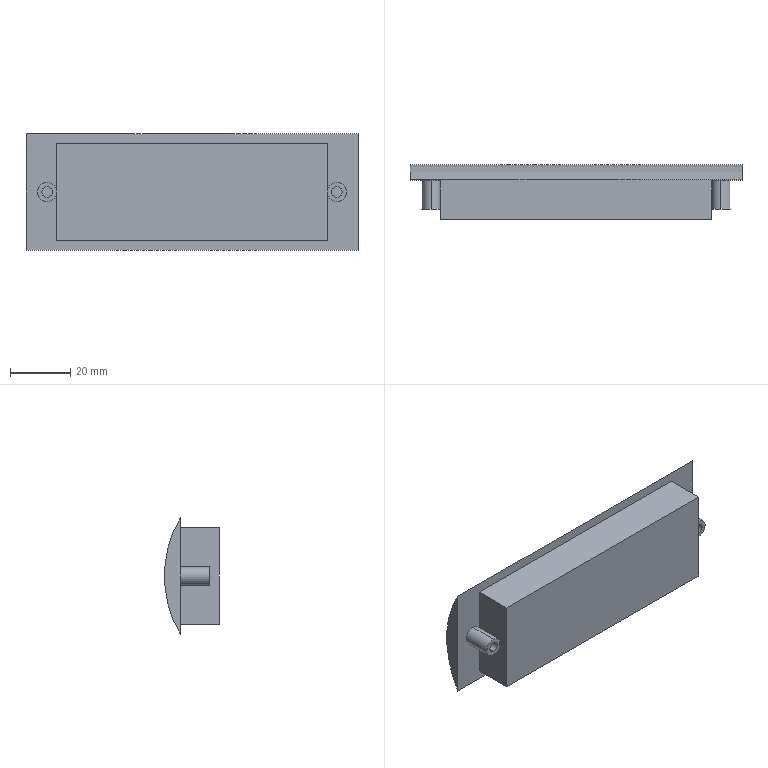Part | STEP file | LE-LLS-96A_LE0314002343 | 1 solid | 23 faces | box 110 x 18.2 x 38.5 mm | volume 52750 mm3 | plane 12 | cylinder 11 | commonest cylinder face diameters 6.3 x6 3.5 x4 76.462 x1
STEP:
#1=CARTESIAN_POINT('',(48.,-9.75,3.15));
#2=VERTEX_POINT('',#1);
#3=CARTESIAN_POINT('',(48.,-9.75,-3.15));
#4=VERTEX_POINT('',#3);
#5=CARTESIAN_POINT('',(48.,-9.75,0.));
#6=DIRECTION('',(0.,1.,0.));
#7=DIRECTION('',(0.,0.,1.));
#8=AXIS2_PLACEMENT_3D('',#5,#6,#7);
#9=CIRCLE('',#8,3.15);
#10=EDGE_CURVE('',#2,#4,#9,.T.);
#11=ORIENTED_EDGE('',*,*,#10,.T.);
#12=CARTESIAN_POINT('',(48.,0.,-3.15));
#13=VERTEX_POINT('',#12);
#14=CARTESIAN_POINT('',(48.,-9.75,-3.15));
#15=DIRECTION('',(0.,1.,0.));
#16=VECTOR('',#15,1000.);
#17=LINE('',#14,#16);
#18=EDGE_CURVE('',#4,#13,#17,.T.);
#19=ORIENTED_EDGE('',*,*,#18,.T.);
#20=CARTESIAN_POINT('',(48.,0.,3.15));
#21=VERTEX_POINT('',#20);
#22=CARTESIAN_POINT('',(48.,0.,0.));
#23=DIRECTION('',(0.,1.,0.));
#24=DIRECTION('',(0.,0.,1.));
#25=AXIS2_PLACEMENT_3D('',#22,#23,#24);
#26=CIRCLE('',#25,3.15);
#27=EDGE_CURVE('',#21,#13,#26,.T.);
#28=ORIENTED_EDGE('',*,*,#27,.F.);
#29=CARTESIAN_POINT('',(48.,-9.75,3.15));
#30=DIRECTION('',(0.,1.,0.));
#31=VECTOR('',#30,1000.);
#32=LINE('',#29,#31);
#33=EDGE_CURVE('',#2,#21,#32,.T.);
#34=ORIENTED_EDGE('',*,*,#33,.F.);
#35=EDGE_LOOP('',(#11,#19,#28,#34));
#36=FACE_OUTER_BOUND('',#35,.T.);
#37=CARTESIAN_POINT('',(48.,-9.75,0.));
#38=DIRECTION('',(0.,1.,0.));
#39=DIRECTION('',(0.,0.,1.));
#40=AXIS2_PLACEMENT_3D('',#37,#38,#39);
#41=CYLINDRICAL_SURFACE('',#40,3.15);
#42=ADVANCED_FACE('',(#36),#41,.T.);
#43=CARTESIAN_POINT('',(45.,-9.75,0.9605));
#44=VERTEX_POINT('',#43);
#45=CARTESIAN_POINT('',(48.,-9.75,0.));
#46=DIRECTION('',(0.,1.,0.));
#47=DIRECTION('',(0.,0.,1.));
#48=AXIS2_PLACEMENT_3D('',#45,#46,#47);
#49=CIRCLE('',#48,3.15);
#50=EDGE_CURVE('',#44,#2,#49,.T.);
#51=ORIENTED_EDGE('',*,*,#50,.T.);
#52=ORIENTED_EDGE('',*,*,#33,.T.);
#53=CARTESIAN_POINT('',(45.,0.,0.9605));
#54=VERTEX_POINT('',#53);
#55=CARTESIAN_POINT('',(48.,0.,0.));
#56=DIRECTION('',(0.,1.,0.));
#57=DIRECTION('',(0.,0.,1.));
#58=AXIS2_PLACEMENT_3D('',#55,#56,#57);
#59=CIRCLE('',#58,3.15);
#60=EDGE_CURVE('',#54,#21,#59,.T.);
#61=ORIENTED_EDGE('',*,*,#60,.F.);
#62=CARTESIAN_POINT('',(45.,-13.,0.9605));
#63=DIRECTION('',(0.,-1.,0.));
#64=VECTOR('',#63,1000.);
#65=LINE('',#62,#64);
#66=EDGE_CURVE('',#54,#44,#65,.T.);
#67=ORIENTED_EDGE('',*,*,#66,.T.);
#68=EDGE_LOOP('',(#51,#52,#61,#67));
#69=FACE_OUTER_BOUND('',#68,.T.);
#70=CARTESIAN_POINT('',(48.,-9.75,0.));
#71=DIRECTION('',(0.,1.,0.));
#72=DIRECTION('',(0.,0.,1.));
#73=AXIS2_PLACEMENT_3D('',#70,#71,#72);
#74=CYLINDRICAL_SURFACE('',#73,3.15);
#75=ADVANCED_FACE('',(#69),#74,.T.);
#76=CARTESIAN_POINT('',(-45.,-9.75,-0.9605));
#77=VERTEX_POINT('',#76);
#78=CARTESIAN_POINT('',(-48.,-9.75,-3.15));
#79=VERTEX_POINT('',#78);
#80=CARTESIAN_POINT('',(-48.,-9.75,0.));
#81=DIRECTION('',(0.,1.,0.));
#82=DIRECTION('',(0.,0.,1.));
#83=AXIS2_PLACEMENT_3D('',#80,#81,#82);
#84=CIRCLE('',#83,3.15);
#85=EDGE_CURVE('',#77,#79,#84,.T.);
#86=ORIENTED_EDGE('',*,*,#85,.T.);
#87=CARTESIAN_POINT('',(-48.,0.,-3.15));
#88=VERTEX_POINT('',#87);
#89=CARTESIAN_POINT('',(-48.,-9.75,-3.15));
#90=DIRECTION('',(0.,1.,0.));
#91=VECTOR('',#90,1000.);
#92=LINE('',#89,#91);
#93=EDGE_CURVE('',#79,#88,#92,.T.);
#94=ORIENTED_EDGE('',*,*,#93,.T.);
#95=CARTESIAN_POINT('',(-45.,0.,-0.9605));
#96=VERTEX_POINT('',#95);
#97=CARTESIAN_POINT('',(-48.,0.,0.));
#98=DIRECTION('',(0.,1.,0.));
#99=DIRECTION('',(0.,0.,1.));
#100=AXIS2_PLACEMENT_3D('',#97,#98,#99);
#101=CIRCLE('',#100,3.15);
#102=EDGE_CURVE('',#96,#88,#101,.T.);
#103=ORIENTED_EDGE('',*,*,#102,.F.);
#104=CARTESIAN_POINT('',(-45.,-13.,-0.9605));
#105=DIRECTION('',(0.,-1.,0.));
#106=VECTOR('',#105,1000.);
#107=LINE('',#104,#106);
#108=EDGE_CURVE('',#96,#77,#107,.T.);
#109=ORIENTED_EDGE('',*,*,#108,.T.);
#110=EDGE_LOOP('',(#86,#94,#103,#109));
#111=FACE_OUTER_BOUND('',#110,.T.);
#112=CARTESIAN_POINT('',(-48.,-9.75,0.));
#113=DIRECTION('',(0.,1.,0.));
#114=DIRECTION('',(0.,0.,1.));
#115=AXIS2_PLACEMENT_3D('',#112,#113,#114);
#116=CYLINDRICAL_SURFACE('',#115,3.15);
#117=ADVANCED_FACE('',(#111),#116,.T.);
#118=ORIENTED_EDGE('',*,*,#93,.F.);
#119=CARTESIAN_POINT('',(-48.,-9.75,3.15));
#120=VERTEX_POINT('',#119);
#121=CARTESIAN_POINT('',(-48.,-9.75,0.));
#122=DIRECTION('',(0.,1.,0.));
#123=DIRECTION('',(0.,0.,1.));
#124=AXIS2_PLACEMENT_3D('',#121,#122,#123);
#125=CIRCLE('',#124,3.15);
#126=EDGE_CURVE('',#79,#120,#125,.T.);
#127=ORIENTED_EDGE('',*,*,#126,.T.);
#128=CARTESIAN_POINT('',(-48.,0.,3.15));
#129=VERTEX_POINT('',#128);
#130=CARTESIAN_POINT('',(-48.,-9.75,3.15));
#131=DIRECTION('',(0.,1.,0.));
#132=VECTOR('',#131,1000.);
#133=LINE('',#130,#132);
#134=EDGE_CURVE('',#120,#129,#133,.T.);
#135=ORIENTED_EDGE('',*,*,#134,.T.);
#136=CARTESIAN_POINT('',(-48.,0.,0.));
#137=DIRECTION('',(0.,1.,0.));
#138=DIRECTION('',(0.,0.,1.));
#139=AXIS2_PLACEMENT_3D('',#136,#137,#138);
#140=CIRCLE('',#139,3.15);
#141=EDGE_CURVE('',#88,#129,#140,.T.);
#142=ORIENTED_EDGE('',*,*,#141,.F.);
#143=EDGE_LOOP('',(#118,#127,#135,#142));
#144=FACE_OUTER_BOUND('',#143,.T.);
#145=CARTESIAN_POINT('',(-48.,-9.75,0.));
#146=DIRECTION('',(0.,1.,0.));
#147=DIRECTION('',(0.,0.,1.));
#148=AXIS2_PLACEMENT_3D('',#145,#146,#147);
#149=CYLINDRICAL_SURFACE('',#148,3.15);
#150=ADVANCED_FACE('',(#144),#149,.T.);
#151=CARTESIAN_POINT('',(48.,0.,1.75));
#152=VERTEX_POINT('',#151);
#153=CARTESIAN_POINT('',(48.,0.,-1.75));
#154=VERTEX_POINT('',#153);
#155=CARTESIAN_POINT('',(48.,0.,0.));
#156=DIRECTION('',(0.,-1.,0.));
#157=DIRECTION('',(0.,0.,-1.));
#158=AXIS2_PLACEMENT_3D('',#155,#156,#157);
#159=CIRCLE('',#158,1.75);
#160=EDGE_CURVE('',#152,#154,#159,.T.);
#161=ORIENTED_EDGE('',*,*,#160,.F.);
#162=CARTESIAN_POINT('',(48.,-9.75,1.75));
#163=VERTEX_POINT('',#162);
#164=CARTESIAN_POINT('',(48.,0.,1.75));
#165=DIRECTION('',(0.,-1.,0.));
#166=VECTOR('',#165,1000.);
#167=LINE('',#164,#166);
#168=EDGE_CURVE('',#152,#163,#167,.T.);
#169=ORIENTED_EDGE('',*,*,#168,.T.);
#170=CARTESIAN_POINT('',(48.,-9.75,-1.75));
#171=VERTEX_POINT('',#170);
#172=CARTESIAN_POINT('',(48.,-9.75,0.));
#173=DIRECTION('',(0.,1.,0.));
#174=DIRECTION('',(0.,0.,-1.));
#175=AXIS2_PLACEMENT_3D('',#172,#173,#174);
#176=CIRCLE('',#175,1.75);
#177=EDGE_CURVE('',#171,#163,#176,.T.);
#178=ORIENTED_EDGE('',*,*,#177,.F.);
#179=CARTESIAN_POINT('',(48.,0.,-1.75));
#180=DIRECTION('',(0.,-1.,0.));
#181=VECTOR('',#180,1000.);
#182=LINE('',#179,#181);
#183=EDGE_CURVE('',#154,#171,#182,.T.);
#184=ORIENTED_EDGE('',*,*,#183,.F.);
#185=EDGE_LOOP('',(#161,#169,#178,#184));
#186=FACE_OUTER_BOUND('',#185,.T.);
#187=CARTESIAN_POINT('',(48.,0.,0.));
#188=DIRECTION('',(0.,-1.,0.));
#189=DIRECTION('',(0.,0.,-1.));
#190=AXIS2_PLACEMENT_3D('',#187,#188,#189);
#191=CYLINDRICAL_SURFACE('',#190,1.75);
#192=ADVANCED_FACE('',(#186),#191,.F.);
#193=CARTESIAN_POINT('',(-48.,0.,1.75));
#194=VERTEX_POINT('',#193);
#195=CARTESIAN_POINT('',(-48.,0.,-1.75));
#196=VERTEX_POINT('',#195);
#197=CARTESIAN_POINT('',(-48.,0.,0.));
#198=DIRECTION('',(0.,-1.,0.));
#199=DIRECTION('',(0.,0.,-1.));
#200=AXIS2_PLACEMENT_3D('',#197,#198,#199);
#201=CIRCLE('',#200,1.75);
#202=EDGE_CURVE('',#194,#196,#201,.T.);
#203=ORIENTED_EDGE('',*,*,#202,.F.);
#204=CARTESIAN_POINT('',(-48.,-9.75,1.75));
#205=VERTEX_POINT('',#204);
#206=CARTESIAN_POINT('',(-48.,0.,1.75));
#207=DIRECTION('',(0.,-1.,0.));
#208=VECTOR('',#207,1000.);
#209=LINE('',#206,#208);
#210=EDGE_CURVE('',#194,#205,#209,.T.);
#211=ORIENTED_EDGE('',*,*,#210,.T.);
#212=CARTESIAN_POINT('',(-48.,-9.75,-1.75));
#213=VERTEX_POINT('',#212);
#214=CARTESIAN_POINT('',(-48.,-9.75,0.));
#215=DIRECTION('',(0.,1.,0.));
#216=DIRECTION('',(0.,0.,-1.));
#217=AXIS2_PLACEMENT_3D('',#214,#215,#216);
#218=CIRCLE('',#217,1.75);
#219=EDGE_CURVE('',#213,#205,#218,.T.);
#220=ORIENTED_EDGE('',*,*,#219,.F.);
#221=CARTESIAN_POINT('',(-48.,0.,-1.75));
#222=DIRECTION('',(0.,-1.,0.));
#223=VECTOR('',#222,1000.);
#224=LINE('',#221,#223);
#225=EDGE_CURVE('',#196,#213,#224,.T.);
#226=ORIENTED_EDGE('',*,*,#225,.F.);
#227=EDGE_LOOP('',(#203,#211,#220,#226));
#228=FACE_OUTER_BOUND('',#227,.T.);
#229=CARTESIAN_POINT('',(-48.,0.,0.));
#230=DIRECTION('',(0.,-1.,0.));
#231=DIRECTION('',(0.,0.,-1.));
#232=AXIS2_PLACEMENT_3D('',#229,#230,#231);
#233=CYLINDRICAL_SURFACE('',#232,1.75);
#234=ADVANCED_FACE('',(#228),#233,.F.);
#235=CARTESIAN_POINT('',(55.,0.,-19.25));
#236=VERTEX_POINT('',#235);
#237=CARTESIAN_POINT('',(-55.,0.,-19.25));
#238=VERTEX_POINT('',#237);
#239=CARTESIAN_POINT('',(55.,0.,-19.25));
#240=DIRECTION('',(-1.,0.,0.));
#241=VECTOR('',#240,1000.);
#242=LINE('',#239,#241);
#243=EDGE_CURVE('',#236,#238,#242,.T.);
#244=ORIENTED_EDGE('',*,*,#243,.T.);
#245=CARTESIAN_POINT('',(-55.,0.,19.25));
#246=VERTEX_POINT('',#245);
#247=CARTESIAN_POINT('',(-55.,-33.031,0.));
#248=DIRECTION('',(1.,0.,0.));
#249=DIRECTION('',(0.,-1.,0.));
#250=AXIS2_PLACEMENT_3D('',#247,#248,#249);
#251=CIRCLE('',#250,38.231);
#252=EDGE_CURVE('',#238,#246,#251,.T.);
#253=ORIENTED_EDGE('',*,*,#252,.T.);
#254=CARTESIAN_POINT('',(55.,0.,19.25));
#255=VERTEX_POINT('',#254);
#256=CARTESIAN_POINT('',(55.,0.,19.25));
#257=DIRECTION('',(1.,0.,0.));
#258=VECTOR('',#257,1000.);
#259=LINE('',#256,#258);
#260=EDGE_CURVE('',#246,#255,#259,.T.);
#261=ORIENTED_EDGE('',*,*,#260,.T.);
#262=CARTESIAN_POINT('',(55.,-33.031,0.));
#263=DIRECTION('',(-1.,0.,0.));
#264=DIRECTION('',(0.,-1.,0.));
#265=AXIS2_PLACEMENT_3D('',#262,#263,#264);
#266=CIRCLE('',#265,38.231);
#267=EDGE_CURVE('',#255,#236,#266,.T.);
#268=ORIENTED_EDGE('',*,*,#267,.T.);
#269=EDGE_LOOP('',(#244,#253,#261,#268));
#270=FACE_OUTER_BOUND('',#269,.T.);
#271=CARTESIAN_POINT('',(55.,-33.031,0.));
#272=DIRECTION('',(-1.,0.,0.));
#273=DIRECTION('',(0.,-1.,0.));
#274=AXIS2_PLACEMENT_3D('',#271,#272,#273);
#275=CYLINDRICAL_SURFACE('',#274,38.231);
#276=ADVANCED_FACE('',(#270),#275,.T.);
#277=ORIENTED_EDGE('',*,*,#252,.F.);
#278=CARTESIAN_POINT('',(-55.,0.,0.));
#279=DIRECTION('',(0.,0.,1.));
#280=VECTOR('',#279,1000.);
#281=LINE('',#278,#280);
#282=EDGE_CURVE('',#238,#246,#281,.T.);
#283=ORIENTED_EDGE('',*,*,#282,.T.);
#284=EDGE_LOOP('',(#277,#283));
#285=FACE_OUTER_BOUND('',#284,.T.);
#286=CARTESIAN_POINT('',(-55.,-33.031,0.));
#287=DIRECTION('',(-1.,0.,0.));
#288=DIRECTION('',(0.,0.,1.));
#289=AXIS2_PLACEMENT_3D('',#286,#287,#288);
#290=PLANE('',#289);
#291=ADVANCED_FACE('',(#285),#290,.T.);
#292=ORIENTED_EDGE('',*,*,#60,.T.);
#293=ORIENTED_EDGE('',*,*,#27,.T.);
#294=CARTESIAN_POINT('',(45.,0.,-0.9605));
#295=VERTEX_POINT('',#294);
#296=CARTESIAN_POINT('',(48.,0.,0.));
#297=DIRECTION('',(0.,1.,0.));
#298=DIRECTION('',(0.,0.,1.));
#299=AXIS2_PLACEMENT_3D('',#296,#297,#298);
#300=CIRCLE('',#299,3.15);
#301=EDGE_CURVE('',#13,#295,#300,.T.);
#302=ORIENTED_EDGE('',*,*,#301,.T.);
#303=CARTESIAN_POINT('',(45.,0.,-16.));
#304=VERTEX_POINT('',#303);
#305=CARTESIAN_POINT('',(45.,0.,-19.25));
#306=DIRECTION('',(0.,0.,-1.));
#307=VECTOR('',#306,1000.);
#308=LINE('',#305,#307);
#309=EDGE_CURVE('',#295,#304,#308,.T.);
#310=ORIENTED_EDGE('',*,*,#309,.T.);
#311=CARTESIAN_POINT('',(-45.,0.,-16.));
#312=VERTEX_POINT('',#311);
#313=CARTESIAN_POINT('',(55.,0.,-16.));
#314=DIRECTION('',(-1.,0.,0.));
#315=VECTOR('',#314,1000.);
#316=LINE('',#313,#315);
#317=EDGE_CURVE('',#304,#312,#316,.T.);
#318=ORIENTED_EDGE('',*,*,#317,.T.);
#319=CARTESIAN_POINT('',(-45.,0.,-19.25));
#320=DIRECTION('',(0.,0.,1.));
#321=VECTOR('',#320,1000.);
#322=LINE('',#319,#321);
#323=EDGE_CURVE('',#312,#96,#322,.T.);
#324=ORIENTED_EDGE('',*,*,#323,.T.);
#325=ORIENTED_EDGE('',*,*,#102,.T.);
#326=ORIENTED_EDGE('',*,*,#141,.T.);
#327=CARTESIAN_POINT('',(-45.,0.,0.9605));
#328=VERTEX_POINT('',#327);
#329=CARTESIAN_POINT('',(-48.,0.,0.));
#330=DIRECTION('',(0.,1.,0.));
#331=DIRECTION('',(0.,0.,1.));
#332=AXIS2_PLACEMENT_3D('',#329,#330,#331);
#333=CIRCLE('',#332,3.15);
#334=EDGE_CURVE('',#129,#328,#333,.T.);
#335=ORIENTED_EDGE('',*,*,#334,.T.);
#336=CARTESIAN_POINT('',(-45.,0.,16.));
#337=VERTEX_POINT('',#336);
#338=CARTESIAN_POINT('',(-45.,0.,-19.25));
#339=DIRECTION('',(0.,0.,1.));
#340=VECTOR('',#339,1000.);
#341=LINE('',#338,#340);
#342=EDGE_CURVE('',#328,#337,#341,.T.);
#343=ORIENTED_EDGE('',*,*,#342,.T.);
#344=CARTESIAN_POINT('',(45.,0.,16.));
#345=VERTEX_POINT('',#344);
#346=CARTESIAN_POINT('',(55.,0.,16.));
#347=DIRECTION('',(1.,0.,0.));
#348=VECTOR('',#347,1000.);
#349=LINE('',#346,#348);
#350=EDGE_CURVE('',#337,#345,#349,.T.);
#351=ORIENTED_EDGE('',*,*,#350,.T.);
#352=CARTESIAN_POINT('',(45.,0.,-19.25));
#353=DIRECTION('',(0.,0.,-1.));
#354=VECTOR('',#353,1000.);
#355=LINE('',#352,#354);
#356=EDGE_CURVE('',#345,#54,#355,.T.);
#357=ORIENTED_EDGE('',*,*,#356,.T.);
#358=EDGE_LOOP('',(#292,#293,#302,#310,#318,#324,#325,#326,#335,#343,#351,#357));
#359=FACE_BOUND('',#358,.T.);
#360=ORIENTED_EDGE('',*,*,#260,.F.);
#361=ORIENTED_EDGE('',*,*,#282,.F.);
#362=ORIENTED_EDGE('',*,*,#243,.F.);
#363=CARTESIAN_POINT('',(55.,0.,-19.25));
#364=DIRECTION('',(0.,0.,1.));
#365=VECTOR('',#364,1000.);
#366=LINE('',#363,#365);
#367=EDGE_CURVE('',#236,#255,#366,.T.);
#368=ORIENTED_EDGE('',*,*,#367,.T.);
#369=EDGE_LOOP('',(#360,#361,#362,#368));
#370=FACE_OUTER_BOUND('',#369,.T.);
#371=CARTESIAN_POINT('',(55.,0.,-19.25));
#372=DIRECTION('',(0.,-1.,0.));
#373=DIRECTION('',(1.,0.,0.));
#374=AXIS2_PLACEMENT_3D('',#371,#372,#373);
#375=PLANE('',#374);
#376=ADVANCED_FACE('',(#359,#370),#375,.T.);
#377=ORIENTED_EDGE('',*,*,#267,.F.);
#378=ORIENTED_EDGE('',*,*,#367,.F.);
#379=EDGE_LOOP('',(#377,#378));
#380=FACE_OUTER_BOUND('',#379,.T.);
#381=CARTESIAN_POINT('',(55.,-33.031,0.));
#382=DIRECTION('',(-1.,0.,0.));
#383=DIRECTION('',(0.,0.,1.));
#384=AXIS2_PLACEMENT_3D('',#381,#382,#383);
#385=PLANE('',#384);
#386=ADVANCED_FACE('',(#380),#385,.F.);
#387=CARTESIAN_POINT('',(45.,-13.,16.));
#388=VERTEX_POINT('',#387);
#389=CARTESIAN_POINT('',(45.,-13.,16.));
#390=DIRECTION('',(0.,1.,0.));
#391=VECTOR('',#390,1000.);
#392=LINE('',#389,#391);
#393=EDGE_CURVE('',#388,#345,#392,.T.);
#394=ORIENTED_EDGE('',*,*,#393,.F.);
#395=CARTESIAN_POINT('',(45.,-13.,-16.));
#396=VERTEX_POINT('',#395);
#397=CARTESIAN_POINT('',(45.,-13.,-16.));
#398=DIRECTION('',(0.,0.,1.));
#399=VECTOR('',#398,1000.);
#400=LINE('',#397,#399);
#401=EDGE_CURVE('',#396,#388,#400,.T.);
#402=ORIENTED_EDGE('',*,*,#401,.F.);
#403=CARTESIAN_POINT('',(45.,-13.,-16.));
#404=DIRECTION('',(0.,-1.,0.));
#405=VECTOR('',#404,1000.);
#406=LINE('',#403,#405);
#407=EDGE_CURVE('',#304,#396,#406,.T.);
#408=ORIENTED_EDGE('',*,*,#407,.F.);
#409=ORIENTED_EDGE('',*,*,#309,.F.);
#410=CARTESIAN_POINT('',(45.,-9.75,-0.9605));
#411=VERTEX_POINT('',#410);
#412=CARTESIAN_POINT('',(45.,-13.,-0.9605));
#413=DIRECTION('',(0.,1.,0.));
#414=VECTOR('',#413,1000.);
#415=LINE('',#412,#414);
#416=EDGE_CURVE('',#411,#295,#415,.T.);
#417=ORIENTED_EDGE('',*,*,#416,.F.);
#418=CARTESIAN_POINT('',(45.,-9.75,-16.));
#419=DIRECTION('',(0.,0.,-1.));
#420=VECTOR('',#419,1000.);
#421=LINE('',#418,#420);
#422=EDGE_CURVE('',#44,#411,#421,.T.);
#423=ORIENTED_EDGE('',*,*,#422,.F.);
#424=ORIENTED_EDGE('',*,*,#66,.F.);
#425=ORIENTED_EDGE('',*,*,#356,.F.);
#426=EDGE_LOOP('',(#394,#402,#408,#409,#417,#423,#424,#425));
#427=FACE_OUTER_BOUND('',#426,.T.);
#428=CARTESIAN_POINT('',(45.,-13.,-16.));
#429=DIRECTION('',(-1.,0.,0.));
#430=DIRECTION('',(0.,0.,1.));
#431=AXIS2_PLACEMENT_3D('',#428,#429,#430);
#432=PLANE('',#431);
#433=ADVANCED_FACE('',(#427),#432,.F.);
#434=ORIENTED_EDGE('',*,*,#18,.F.);
#435=CARTESIAN_POINT('',(48.,-9.75,0.));
#436=DIRECTION('',(0.,1.,0.));
#437=DIRECTION('',(0.,0.,1.));
#438=AXIS2_PLACEMENT_3D('',#435,#436,#437);
#439=CIRCLE('',#438,3.15);
#440=EDGE_CURVE('',#4,#411,#439,.T.);
#441=ORIENTED_EDGE('',*,*,#440,.T.);
#442=ORIENTED_EDGE('',*,*,#416,.T.);
#443=ORIENTED_EDGE('',*,*,#301,.F.);
#444=EDGE_LOOP('',(#434,#441,#442,#443));
#445=FACE_OUTER_BOUND('',#444,.T.);
#446=CARTESIAN_POINT('',(48.,-9.75,0.));
#447=DIRECTION('',(0.,1.,0.));
#448=DIRECTION('',(0.,0.,1.));
#449=AXIS2_PLACEMENT_3D('',#446,#447,#448);
#450=CYLINDRICAL_SURFACE('',#449,3.15);
#451=ADVANCED_FACE('',(#445),#450,.T.);
#452=CARTESIAN_POINT('',(-45.,-13.,16.));
#453=VERTEX_POINT('',#452);
#454=CARTESIAN_POINT('',(-45.,-13.,16.));
#455=DIRECTION('',(-1.,0.,0.));
#456=VECTOR('',#455,1000.);
#457=LINE('',#454,#456);
#458=EDGE_CURVE('',#388,#453,#457,.T.);
#459=ORIENTED_EDGE('',*,*,#458,.F.);
#460=ORIENTED_EDGE('',*,*,#393,.T.);
#461=ORIENTED_EDGE('',*,*,#350,.F.);
#462=CARTESIAN_POINT('',(-45.,-13.,16.));
#463=DIRECTION('',(0.,1.,0.));
#464=VECTOR('',#463,1000.);
#465=LINE('',#462,#464);
#466=EDGE_CURVE('',#453,#337,#465,.T.);
#467=ORIENTED_EDGE('',*,*,#466,.F.);
#468=EDGE_LOOP('',(#459,#460,#461,#467));
#469=FACE_OUTER_BOUND('',#468,.T.);
#470=CARTESIAN_POINT('',(-45.,-13.,16.));
#471=DIRECTION('',(0.,0.,-1.));
#472=DIRECTION('',(-1.,0.,0.));
#473=AXIS2_PLACEMENT_3D('',#470,#471,#472);
#474=PLANE('',#473);
#475=ADVANCED_FACE('',(#469),#474,.F.);
#476=ORIENTED_EDGE('',*,*,#323,.F.);
#477=CARTESIAN_POINT('',(-45.,-13.,-16.));
#478=VERTEX_POINT('',#477);
#479=CARTESIAN_POINT('',(-45.,-13.,-16.));
#480=DIRECTION('',(0.,1.,0.));
#481=VECTOR('',#480,1000.);
#482=LINE('',#479,#481);
#483=EDGE_CURVE('',#478,#312,#482,.T.);
#484=ORIENTED_EDGE('',*,*,#483,.F.);
#485=CARTESIAN_POINT('',(-45.,-13.,-16.));
#486=DIRECTION('',(0.,0.,-1.));
#487=VECTOR('',#486,1000.);
#488=LINE('',#485,#487);
#489=EDGE_CURVE('',#453,#478,#488,.T.);
#490=ORIENTED_EDGE('',*,*,#489,.F.);
#491=ORIENTED_EDGE('',*,*,#466,.T.);
#492=ORIENTED_EDGE('',*,*,#342,.F.);
#493=CARTESIAN_POINT('',(-45.,-9.75,0.9605));
#494=VERTEX_POINT('',#493);
#495=CARTESIAN_POINT('',(-45.,-13.,0.9605));
#496=DIRECTION('',(0.,1.,0.));
#497=VECTOR('',#496,1000.);
#498=LINE('',#495,#497);
#499=EDGE_CURVE('',#494,#328,#498,.T.);
#500=ORIENTED_EDGE('',*,*,#499,.F.);
#501=CARTESIAN_POINT('',(-45.,-9.75,-16.));
#502=DIRECTION('',(0.,0.,1.));
#503=VECTOR('',#502,1000.);
#504=LINE('',#501,#503);
#505=EDGE_CURVE('',#77,#494,#504,.T.);
#506=ORIENTED_EDGE('',*,*,#505,.F.);
#507=ORIENTED_EDGE('',*,*,#108,.F.);
#508=EDGE_LOOP('',(#476,#484,#490,#491,#492,#500,#506,#507));
#509=FACE_OUTER_BOUND('',#508,.T.);
#510=CARTESIAN_POINT('',(-45.,-13.,-16.));
#511=DIRECTION('',(1.,0.,0.));
#512=DIRECTION('',(0.,0.,-1.));
#513=AXIS2_PLACEMENT_3D('',#510,#511,#512);
#514=PLANE('',#513);
#515=ADVANCED_FACE('',(#509),#514,.F.);
#516=ORIENTED_EDGE('',*,*,#134,.F.);
#517=CARTESIAN_POINT('',(-48.,-9.75,0.));
#518=DIRECTION('',(0.,1.,0.));
#519=DIRECTION('',(0.,0.,1.));
#520=AXIS2_PLACEMENT_3D('',#517,#518,#519);
#521=CIRCLE('',#520,3.15);
#522=EDGE_CURVE('',#120,#494,#521,.T.);
#523=ORIENTED_EDGE('',*,*,#522,.T.);
#524=ORIENTED_EDGE('',*,*,#499,.T.);
#525=ORIENTED_EDGE('',*,*,#334,.F.);
#526=EDGE_LOOP('',(#516,#523,#524,#525));
#527=FACE_OUTER_BOUND('',#526,.T.);
#528=CARTESIAN_POINT('',(-48.,-9.75,0.));
#529=DIRECTION('',(0.,1.,0.));
#530=DIRECTION('',(0.,0.,1.));
#531=AXIS2_PLACEMENT_3D('',#528,#529,#530);
#532=CYLINDRICAL_SURFACE('',#531,3.15);
#533=ADVANCED_FACE('',(#527),#532,.T.);
#534=CARTESIAN_POINT('',(-45.,-13.,-16.));
#535=DIRECTION('',(1.,0.,0.));
#536=VECTOR('',#535,1000.);
#537=LINE('',#534,#536);
#538=EDGE_CURVE('',#478,#396,#537,.T.);
#539=ORIENTED_EDGE('',*,*,#538,.F.);
#540=ORIENTED_EDGE('',*,*,#483,.T.);
#541=ORIENTED_EDGE('',*,*,#317,.F.);
#542=ORIENTED_EDGE('',*,*,#407,.T.);
#543=EDGE_LOOP('',(#539,#540,#541,#542));
#544=FACE_OUTER_BOUND('',#543,.T.);
#545=CARTESIAN_POINT('',(-45.,-13.,-16.));
#546=DIRECTION('',(0.,0.,1.));
#547=DIRECTION('',(1.,0.,0.));
#548=AXIS2_PLACEMENT_3D('',#545,#546,#547);
#549=PLANE('',#548);
#550=ADVANCED_FACE('',(#544),#549,.F.);
#551=ORIENTED_EDGE('',*,*,#538,.T.);
#552=ORIENTED_EDGE('',*,*,#401,.T.);
#553=ORIENTED_EDGE('',*,*,#458,.T.);
#554=ORIENTED_EDGE('',*,*,#489,.T.);
#555=EDGE_LOOP('',(#551,#552,#553,#554));
#556=FACE_OUTER_BOUND('',#555,.T.);
#557=CARTESIAN_POINT('',(45.,-13.,-16.));
#558=DIRECTION('',(0.,-1.,0.));
#559=DIRECTION('',(0.,0.,-1.));
#560=AXIS2_PLACEMENT_3D('',#557,#558,#559);
#561=PLANE('',#560);
#562=ADVANCED_FACE('',(#556),#561,.T.);
#563=ORIENTED_EDGE('',*,*,#177,.T.);
#564=CARTESIAN_POINT('',(48.,-9.75,0.));
#565=DIRECTION('',(0.,1.,0.));
#566=DIRECTION('',(0.,0.,-1.));
#567=AXIS2_PLACEMENT_3D('',#564,#565,#566);
#568=CIRCLE('',#567,1.75);
#569=EDGE_CURVE('',#163,#171,#568,.T.);
#570=ORIENTED_EDGE('',*,*,#569,.T.);
#571=EDGE_LOOP('',(#563,#570));
#572=FACE_BOUND('',#571,.T.);
#573=ORIENTED_EDGE('',*,*,#50,.F.);
#574=ORIENTED_EDGE('',*,*,#422,.T.);
#575=ORIENTED_EDGE('',*,*,#440,.F.);
#576=ORIENTED_EDGE('',*,*,#10,.F.);
#577=EDGE_LOOP('',(#573,#574,#575,#576));
#578=FACE_OUTER_BOUND('',#577,.T.);
#579=CARTESIAN_POINT('',(48.,-9.75,0.));
#580=DIRECTION('',(0.,-1.,0.));
#581=DIRECTION('',(1.,0.,0.));
#582=AXIS2_PLACEMENT_3D('',#579,#580,#581);
#583=PLANE('',#582);
#584=ADVANCED_FACE('',(#572,#578),#583,.T.);
#585=ORIENTED_EDGE('',*,*,#85,.F.);
#586=ORIENTED_EDGE('',*,*,#505,.T.);
#587=ORIENTED_EDGE('',*,*,#522,.F.);
#588=ORIENTED_EDGE('',*,*,#126,.F.);
#589=EDGE_LOOP('',(#585,#586,#587,#588));
#590=FACE_OUTER_BOUND('',#589,.T.);
#591=ORIENTED_EDGE('',*,*,#219,.T.);
#592=CARTESIAN_POINT('',(-48.,-9.75,0.));
#593=DIRECTION('',(0.,1.,0.));
#594=DIRECTION('',(0.,0.,-1.));
#595=AXIS2_PLACEMENT_3D('',#592,#593,#594);
#596=CIRCLE('',#595,1.75);
#597=EDGE_CURVE('',#205,#213,#596,.T.);
#598=ORIENTED_EDGE('',*,*,#597,.T.);
#599=EDGE_LOOP('',(#591,#598));
#600=FACE_BOUND('',#599,.T.);
#601=CARTESIAN_POINT('',(-48.,-9.75,0.));
#602=DIRECTION('',(0.,-1.,0.));
#603=DIRECTION('',(1.,0.,0.));
#604=AXIS2_PLACEMENT_3D('',#601,#602,#603);
#605=PLANE('',#604);
#606=ADVANCED_FACE('',(#590,#600),#605,.T.);
#607=ORIENTED_EDGE('',*,*,#168,.F.);
#608=CARTESIAN_POINT('',(48.,0.,0.));
#609=DIRECTION('',(0.,-1.,0.));
#610=DIRECTION('',(0.,0.,-1.));
#611=AXIS2_PLACEMENT_3D('',#608,#609,#610);
#612=CIRCLE('',#611,1.75);
#613=EDGE_CURVE('',#154,#152,#612,.T.);
#614=ORIENTED_EDGE('',*,*,#613,.F.);
#615=ORIENTED_EDGE('',*,*,#183,.T.);
#616=ORIENTED_EDGE('',*,*,#569,.F.);
#617=EDGE_LOOP('',(#607,#614,#615,#616));
#618=FACE_OUTER_BOUND('',#617,.T.);
#619=CARTESIAN_POINT('',(48.,0.,0.));
#620=DIRECTION('',(0.,-1.,0.));
#621=DIRECTION('',(0.,0.,-1.));
#622=AXIS2_PLACEMENT_3D('',#619,#620,#621);
#623=CYLINDRICAL_SURFACE('',#622,1.75);
#624=ADVANCED_FACE('',(#618),#623,.F.);
#625=ORIENTED_EDGE('',*,*,#210,.F.);
#626=CARTESIAN_POINT('',(-48.,0.,0.));
#627=DIRECTION('',(0.,-1.,0.));
#628=DIRECTION('',(0.,0.,-1.));
#629=AXIS2_PLACEMENT_3D('',#626,#627,#628);
#630=CIRCLE('',#629,1.75);
#631=EDGE_CURVE('',#196,#194,#630,.T.);
#632=ORIENTED_EDGE('',*,*,#631,.F.);
#633=ORIENTED_EDGE('',*,*,#225,.T.);
#634=ORIENTED_EDGE('',*,*,#597,.F.);
#635=EDGE_LOOP('',(#625,#632,#633,#634));
#636=FACE_OUTER_BOUND('',#635,.T.);
#637=CARTESIAN_POINT('',(-48.,0.,0.));
#638=DIRECTION('',(0.,-1.,0.));
#639=DIRECTION('',(0.,0.,-1.));
#640=AXIS2_PLACEMENT_3D('',#637,#638,#639);
#641=CYLINDRICAL_SURFACE('',#640,1.75);
#642=ADVANCED_FACE('',(#636),#641,.F.);
#643=ORIENTED_EDGE('',*,*,#613,.T.);
#644=ORIENTED_EDGE('',*,*,#160,.T.);
#645=EDGE_LOOP('',(#643,#644));
#646=FACE_OUTER_BOUND('',#645,.T.);
#647=CARTESIAN_POINT('',(48.,0.,0.));
#648=DIRECTION('',(0.,-1.,0.));
#649=DIRECTION('',(1.,0.,0.));
#650=AXIS2_PLACEMENT_3D('',#647,#648,#649);
#651=PLANE('',#650);
#652=ADVANCED_FACE('',(#646),#651,.T.);
#653=ORIENTED_EDGE('',*,*,#631,.T.);
#654=ORIENTED_EDGE('',*,*,#202,.T.);
#655=EDGE_LOOP('',(#653,#654));
#656=FACE_OUTER_BOUND('',#655,.T.);
#657=CARTESIAN_POINT('',(-48.,0.,0.));
#658=DIRECTION('',(0.,-1.,0.));
#659=DIRECTION('',(1.,0.,0.));
#660=AXIS2_PLACEMENT_3D('',#657,#658,#659);
#661=PLANE('',#660);
#662=ADVANCED_FACE('',(#656),#661,.T.);
#663=CLOSED_SHELL('',(#42,#75,#117,#150,#192,#234,#276,#291,#376,#386,#433,#451,#475,#515,#533,#550,#562,#584,#606,#624,#642,#652,#662));
#664=MANIFOLD_SOLID_BREP('',#663);
#665=CARTESIAN_POINT('',(0.,0.,0.));
#666=DIRECTION('',(0.,0.,1.));
#667=DIRECTION('',(1.,0.,0.));
#668=AXIS2_PLACEMENT_3D('',#665,#666,#667);
#669=(LENGTH_UNIT()NAMED_UNIT(*)SI_UNIT(.MILLI.,.METRE.));
#670=UNCERTAINTY_MEASURE_WITH_UNIT(LENGTH_MEASURE(0.00001),#669,'','');
#671=(NAMED_UNIT(*)PLANE_ANGLE_UNIT()SI_UNIT($,.RADIAN.));
#672=(NAMED_UNIT(*)SI_UNIT($,.STERADIAN.)SOLID_ANGLE_UNIT());
#673=(GEOMETRIC_REPRESENTATION_CONTEXT(3)GLOBAL_UNCERTAINTY_ASSIGNED_CONTEXT((#670))GLOBAL_UNIT_ASSIGNED_CONTEXT((#669,#671,#672))REPRESENTATION_CONTEXT('',''));
#674=ADVANCED_BREP_SHAPE_REPRESENTATION('',(#664,#668),#673);